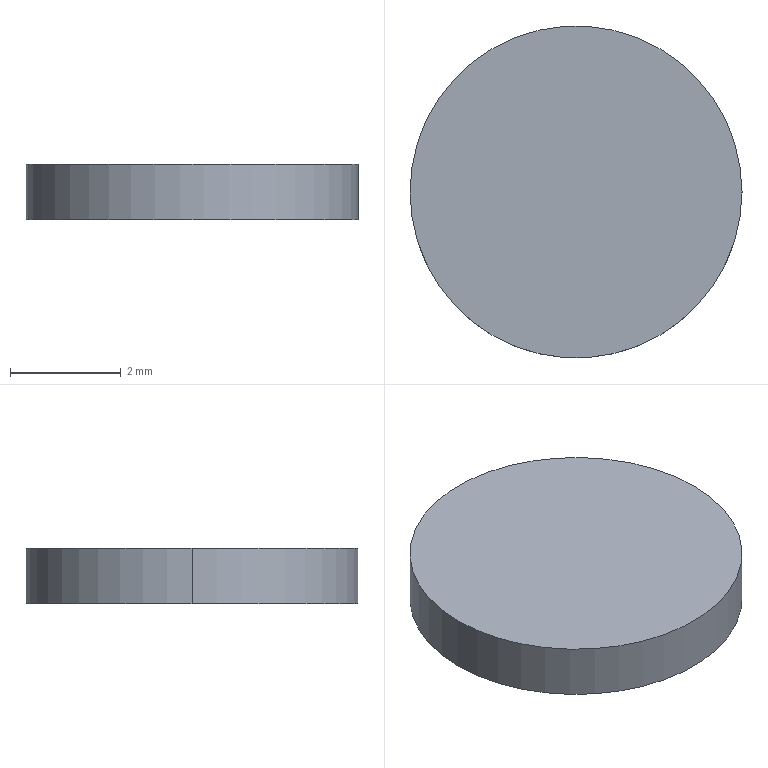Part | STEP file | 1 solid | 4 faces | box 6 x 6 x 1 mm | volume 28.274 mm3 | plane 2 | cylinder 2 | commonest cylinder face diameters 6 x2
STEP:
#1=CARTESIAN_POINT('',(-3.,0.,0.));
#2=VERTEX_POINT('',#1);
#3=CARTESIAN_POINT('',(3.,0.,0.));
#4=VERTEX_POINT('',#3);
#5=CARTESIAN_POINT('',(0.,0.,0.));
#6=DIRECTION('',(0.,0.,1.));
#7=DIRECTION('',(1.,0.,0.));
#8=AXIS2_PLACEMENT_3D('',#5,#6,#7);
#9=CIRCLE('',#8,3.);
#10=EDGE_CURVE('',#2,#4,#9,.T.);
#11=ORIENTED_EDGE('',*,*,#10,.F.);
#12=CARTESIAN_POINT('',(0.,0.,0.));
#13=DIRECTION('',(0.,0.,1.));
#14=DIRECTION('',(1.,0.,0.));
#15=AXIS2_PLACEMENT_3D('',#12,#13,#14);
#16=CIRCLE('',#15,3.);
#17=EDGE_CURVE('',#4,#2,#16,.T.);
#18=ORIENTED_EDGE('',*,*,#17,.F.);
#19=EDGE_LOOP('',(#11,#18));
#20=FACE_OUTER_BOUND('',#19,.T.);
#21=CARTESIAN_POINT('',(0.,0.,0.));
#22=DIRECTION('',(0.,0.,1.));
#23=DIRECTION('',(1.,0.,0.));
#24=AXIS2_PLACEMENT_3D('',#21,#22,#23);
#25=PLANE('',#24);
#26=ADVANCED_FACE('',(#20),#25,.F.);
#27=CARTESIAN_POINT('',(-3.,0.,1.));
#28=VERTEX_POINT('',#27);
#29=CARTESIAN_POINT('',(3.,0.,1.));
#30=VERTEX_POINT('',#29);
#31=CARTESIAN_POINT('',(0.,0.,1.));
#32=DIRECTION('',(0.,0.,1.));
#33=DIRECTION('',(1.,0.,0.));
#34=AXIS2_PLACEMENT_3D('',#31,#32,#33);
#35=CIRCLE('',#34,3.);
#36=EDGE_CURVE('',#28,#30,#35,.T.);
#37=ORIENTED_EDGE('',*,*,#36,.T.);
#38=CARTESIAN_POINT('',(0.,0.,1.));
#39=DIRECTION('',(0.,0.,1.));
#40=DIRECTION('',(1.,0.,0.));
#41=AXIS2_PLACEMENT_3D('',#38,#39,#40);
#42=CIRCLE('',#41,3.);
#43=EDGE_CURVE('',#30,#28,#42,.T.);
#44=ORIENTED_EDGE('',*,*,#43,.T.);
#45=EDGE_LOOP('',(#37,#44));
#46=FACE_OUTER_BOUND('',#45,.T.);
#47=CARTESIAN_POINT('',(0.,0.,1.));
#48=DIRECTION('',(0.,0.,1.));
#49=DIRECTION('',(1.,0.,0.));
#50=AXIS2_PLACEMENT_3D('',#47,#48,#49);
#51=PLANE('',#50);
#52=ADVANCED_FACE('',(#46),#51,.T.);
#53=CARTESIAN_POINT('',(3.,0.,1.));
#54=DIRECTION('',(0.,0.,-1.));
#55=VECTOR('',#54,1000.);
#56=LINE('',#53,#55);
#57=EDGE_CURVE('',#30,#4,#56,.T.);
#58=ORIENTED_EDGE('',*,*,#57,.F.);
#59=ORIENTED_EDGE('',*,*,#36,.F.);
#60=CARTESIAN_POINT('',(-3.,0.,1.));
#61=DIRECTION('',(0.,0.,-1.));
#62=VECTOR('',#61,1000.);
#63=LINE('',#60,#62);
#64=EDGE_CURVE('',#28,#2,#63,.T.);
#65=ORIENTED_EDGE('',*,*,#64,.T.);
#66=ORIENTED_EDGE('',*,*,#10,.T.);
#67=EDGE_LOOP('',(#58,#59,#65,#66));
#68=FACE_OUTER_BOUND('',#67,.T.);
#69=CARTESIAN_POINT('',(0.,0.,1.));
#70=DIRECTION('',(0.,0.,-1.));
#71=DIRECTION('',(-1.,0.,0.));
#72=AXIS2_PLACEMENT_3D('',#69,#70,#71);
#73=CYLINDRICAL_SURFACE('',#72,3.);
#74=ADVANCED_FACE('',(#68),#73,.T.);
#75=ORIENTED_EDGE('',*,*,#43,.F.);
#76=ORIENTED_EDGE('',*,*,#57,.T.);
#77=ORIENTED_EDGE('',*,*,#17,.T.);
#78=ORIENTED_EDGE('',*,*,#64,.F.);
#79=EDGE_LOOP('',(#75,#76,#77,#78));
#80=FACE_OUTER_BOUND('',#79,.T.);
#81=CARTESIAN_POINT('',(0.,0.,1.));
#82=DIRECTION('',(0.,0.,-1.));
#83=DIRECTION('',(-1.,0.,0.));
#84=AXIS2_PLACEMENT_3D('',#81,#82,#83);
#85=CYLINDRICAL_SURFACE('',#84,3.);
#86=ADVANCED_FACE('',(#80),#85,.T.);
#87=CLOSED_SHELL('',(#26,#52,#74,#86));
#88=MANIFOLD_SOLID_BREP('',#87);
#89=CARTESIAN_POINT('',(0.,0.,0.));
#90=DIRECTION('',(0.,0.,1.));
#91=DIRECTION('',(1.,0.,0.));
#92=AXIS2_PLACEMENT_3D('',#89,#90,#91);
#93=(LENGTH_UNIT()NAMED_UNIT(*)SI_UNIT(.MILLI.,.METRE.));
#94=UNCERTAINTY_MEASURE_WITH_UNIT(LENGTH_MEASURE(0.00001),#93,'','');
#95=(NAMED_UNIT(*)PLANE_ANGLE_UNIT()SI_UNIT($,.RADIAN.));
#96=(NAMED_UNIT(*)SI_UNIT($,.STERADIAN.)SOLID_ANGLE_UNIT());
#97=(GEOMETRIC_REPRESENTATION_CONTEXT(3)GLOBAL_UNCERTAINTY_ASSIGNED_CONTEXT((#94))GLOBAL_UNIT_ASSIGNED_CONTEXT((#93,#95,#96))REPRESENTATION_CONTEXT('',''));
#98=ADVANCED_BREP_SHAPE_REPRESENTATION('',(#88,#92),#97);